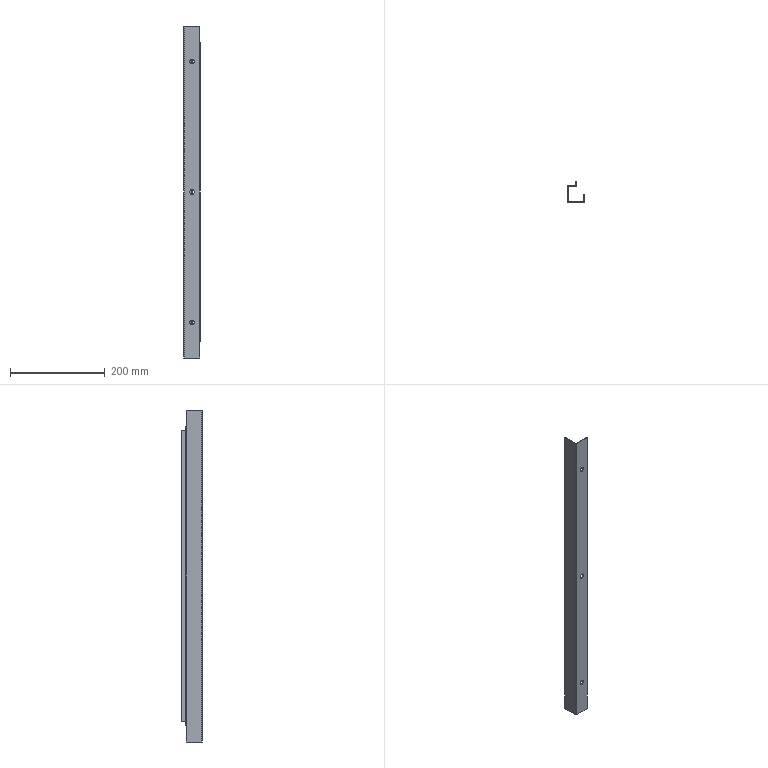Part | SolidWorks | features EdgeFlange 3, ICE 2, FlatPattern 1, LPattern 1, SMBaseFlange 1, SheetMetal 1 | 1 solid | 50 faces | box 35 x 43.5 x 700 mm | volume 106566 mm3 | plane 36 | cylinder 14 | commonest cylinder face diameters 10 x6 3 x4 4.5 x4
STEP:
#1=CARTESIAN_POINT('',(7.75,33.5,307.5));
#2=VERTEX_POINT('',#1);
#3=CARTESIAN_POINT('',(3.25,33.5,307.5));
#4=VERTEX_POINT('',#3);
#5=CARTESIAN_POINT('',(5.5,33.5,307.5));
#6=DIRECTION('',(0.,1.,0.));
#7=DIRECTION('',(-1.,0.,0.));
#8=AXIS2_PLACEMENT_3D('',#5,#6,#7);
#9=CIRCLE('',#8,2.25);
#10=EDGE_CURVE('',#2,#4,#9,.T.);
#11=ORIENTED_EDGE('',*,*,#10,.F.);
#12=CARTESIAN_POINT('',(7.75,35.,307.5));
#13=VERTEX_POINT('',#12);
#14=CARTESIAN_POINT('',(7.75,33.5,307.5));
#15=DIRECTION('',(0.,1.,0.));
#16=VECTOR('',#15,1000.);
#17=LINE('',#14,#16);
#18=EDGE_CURVE('',#2,#13,#17,.T.);
#19=ORIENTED_EDGE('',*,*,#18,.T.);
#20=CARTESIAN_POINT('',(3.25,35.,307.5));
#21=VERTEX_POINT('',#20);
#22=CARTESIAN_POINT('',(5.5,35.,307.5));
#23=DIRECTION('',(0.,1.,0.));
#24=DIRECTION('',(-1.,0.,0.));
#25=AXIS2_PLACEMENT_3D('',#22,#23,#24);
#26=CIRCLE('',#25,2.25);
#27=EDGE_CURVE('',#13,#21,#26,.T.);
#28=ORIENTED_EDGE('',*,*,#27,.T.);
#29=CARTESIAN_POINT('',(3.25,33.5,307.5));
#30=DIRECTION('',(0.,1.,0.));
#31=VECTOR('',#30,1000.);
#32=LINE('',#29,#31);
#33=EDGE_CURVE('',#4,#21,#32,.T.);
#34=ORIENTED_EDGE('',*,*,#33,.F.);
#35=EDGE_LOOP('',(#11,#19,#28,#34));
#36=FACE_OUTER_BOUND('',#35,.T.);
#37=CARTESIAN_POINT('',(5.5,33.5,307.5));
#38=DIRECTION('',(0.,1.,0.));
#39=DIRECTION('',(-1.,0.,0.));
#40=AXIS2_PLACEMENT_3D('',#37,#38,#39);
#41=CYLINDRICAL_SURFACE('',#40,2.25);
#42=ADVANCED_FACE('',(#36),#41,.F.);
#43=CARTESIAN_POINT('',(7.75,33.5,-307.5));
#44=VERTEX_POINT('',#43);
#45=CARTESIAN_POINT('',(3.25,33.5,-307.5));
#46=VERTEX_POINT('',#45);
#47=CARTESIAN_POINT('',(5.5,33.5,-307.5));
#48=DIRECTION('',(0.,1.,0.));
#49=DIRECTION('',(-1.,0.,0.));
#50=AXIS2_PLACEMENT_3D('',#47,#48,#49);
#51=CIRCLE('',#50,2.25);
#52=EDGE_CURVE('',#44,#46,#51,.T.);
#53=ORIENTED_EDGE('',*,*,#52,.F.);
#54=CARTESIAN_POINT('',(7.75,35.,-307.5));
#55=VERTEX_POINT('',#54);
#56=CARTESIAN_POINT('',(7.75,33.5,-307.5));
#57=DIRECTION('',(0.,1.,0.));
#58=VECTOR('',#57,1000.);
#59=LINE('',#56,#58);
#60=EDGE_CURVE('',#44,#55,#59,.T.);
#61=ORIENTED_EDGE('',*,*,#60,.T.);
#62=CARTESIAN_POINT('',(3.25,35.,-307.5));
#63=VERTEX_POINT('',#62);
#64=CARTESIAN_POINT('',(5.5,35.,-307.5));
#65=DIRECTION('',(0.,1.,0.));
#66=DIRECTION('',(-1.,0.,0.));
#67=AXIS2_PLACEMENT_3D('',#64,#65,#66);
#68=CIRCLE('',#67,2.25);
#69=EDGE_CURVE('',#55,#63,#68,.T.);
#70=ORIENTED_EDGE('',*,*,#69,.T.);
#71=CARTESIAN_POINT('',(3.25,33.5,-307.5));
#72=DIRECTION('',(0.,1.,0.));
#73=VECTOR('',#72,1000.);
#74=LINE('',#71,#73);
#75=EDGE_CURVE('',#46,#63,#74,.T.);
#76=ORIENTED_EDGE('',*,*,#75,.F.);
#77=EDGE_LOOP('',(#53,#61,#70,#76));
#78=FACE_OUTER_BOUND('',#77,.T.);
#79=CARTESIAN_POINT('',(5.5,33.5,-307.5));
#80=DIRECTION('',(0.,1.,0.));
#81=DIRECTION('',(-1.,0.,0.));
#82=AXIS2_PLACEMENT_3D('',#79,#80,#81);
#83=CYLINDRICAL_SURFACE('',#82,2.25);
#84=ADVANCED_FACE('',(#78),#83,.F.);
#85=CARTESIAN_POINT('',(17.5,1.5,-270.));
#86=VERTEX_POINT('',#85);
#87=CARTESIAN_POINT('',(17.5,1.5,-280.));
#88=VERTEX_POINT('',#87);
#89=CARTESIAN_POINT('',(17.5,1.5,-275.));
#90=DIRECTION('',(0.,-1.,0.));
#91=DIRECTION('',(0.,0.,-1.));
#92=AXIS2_PLACEMENT_3D('',#89,#90,#91);
#93=CIRCLE('',#92,5.);
#94=EDGE_CURVE('',#86,#88,#93,.T.);
#95=ORIENTED_EDGE('',*,*,#94,.F.);
#96=CARTESIAN_POINT('',(17.5,0.,-270.));
#97=VERTEX_POINT('',#96);
#98=CARTESIAN_POINT('',(17.5,1.5,-270.));
#99=DIRECTION('',(0.,-1.,0.));
#100=VECTOR('',#99,1000.);
#101=LINE('',#98,#100);
#102=EDGE_CURVE('',#86,#97,#101,.T.);
#103=ORIENTED_EDGE('',*,*,#102,.T.);
#104=CARTESIAN_POINT('',(17.5,0.,-280.));
#105=VERTEX_POINT('',#104);
#106=CARTESIAN_POINT('',(17.5,0.,-275.));
#107=DIRECTION('',(0.,-1.,0.));
#108=DIRECTION('',(0.,0.,-1.));
#109=AXIS2_PLACEMENT_3D('',#106,#107,#108);
#110=CIRCLE('',#109,5.);
#111=EDGE_CURVE('',#97,#105,#110,.T.);
#112=ORIENTED_EDGE('',*,*,#111,.T.);
#113=CARTESIAN_POINT('',(17.5,1.5,-280.));
#114=DIRECTION('',(0.,-1.,0.));
#115=VECTOR('',#114,1000.);
#116=LINE('',#113,#115);
#117=EDGE_CURVE('',#88,#105,#116,.T.);
#118=ORIENTED_EDGE('',*,*,#117,.F.);
#119=EDGE_LOOP('',(#95,#103,#112,#118));
#120=FACE_OUTER_BOUND('',#119,.T.);
#121=CARTESIAN_POINT('',(17.5,1.5,-275.));
#122=DIRECTION('',(0.,-1.,0.));
#123=DIRECTION('',(0.,0.,-1.));
#124=AXIS2_PLACEMENT_3D('',#121,#122,#123);
#125=CYLINDRICAL_SURFACE('',#124,5.);
#126=ADVANCED_FACE('',(#120),#125,.F.);
#127=CARTESIAN_POINT('',(17.5,1.5,5.));
#128=VERTEX_POINT('',#127);
#129=CARTESIAN_POINT('',(17.5,1.5,-5.));
#130=VERTEX_POINT('',#129);
#131=CARTESIAN_POINT('',(17.5,1.5,0.));
#132=DIRECTION('',(0.,-1.,0.));
#133=DIRECTION('',(0.,0.,-1.));
#134=AXIS2_PLACEMENT_3D('',#131,#132,#133);
#135=CIRCLE('',#134,5.);
#136=EDGE_CURVE('',#128,#130,#135,.T.);
#137=ORIENTED_EDGE('',*,*,#136,.F.);
#138=CARTESIAN_POINT('',(17.5,0.,5.));
#139=VERTEX_POINT('',#138);
#140=CARTESIAN_POINT('',(17.5,1.5,5.));
#141=DIRECTION('',(0.,-1.,0.));
#142=VECTOR('',#141,1000.);
#143=LINE('',#140,#142);
#144=EDGE_CURVE('',#128,#139,#143,.T.);
#145=ORIENTED_EDGE('',*,*,#144,.T.);
#146=CARTESIAN_POINT('',(17.5,0.,-5.));
#147=VERTEX_POINT('',#146);
#148=CARTESIAN_POINT('',(17.5,0.,0.));
#149=DIRECTION('',(0.,-1.,0.));
#150=DIRECTION('',(0.,0.,-1.));
#151=AXIS2_PLACEMENT_3D('',#148,#149,#150);
#152=CIRCLE('',#151,5.);
#153=EDGE_CURVE('',#139,#147,#152,.T.);
#154=ORIENTED_EDGE('',*,*,#153,.T.);
#155=CARTESIAN_POINT('',(17.5,1.5,-5.));
#156=DIRECTION('',(0.,-1.,0.));
#157=VECTOR('',#156,1000.);
#158=LINE('',#155,#157);
#159=EDGE_CURVE('',#130,#147,#158,.T.);
#160=ORIENTED_EDGE('',*,*,#159,.F.);
#161=EDGE_LOOP('',(#137,#145,#154,#160));
#162=FACE_OUTER_BOUND('',#161,.T.);
#163=CARTESIAN_POINT('',(17.5,1.5,0.));
#164=DIRECTION('',(0.,-1.,0.));
#165=DIRECTION('',(0.,0.,-1.));
#166=AXIS2_PLACEMENT_3D('',#163,#164,#165);
#167=CYLINDRICAL_SURFACE('',#166,5.);
#168=ADVANCED_FACE('',(#162),#167,.F.);
#169=CARTESIAN_POINT('',(17.5,1.5,280.));
#170=VERTEX_POINT('',#169);
#171=CARTESIAN_POINT('',(17.5,1.5,270.));
#172=VERTEX_POINT('',#171);
#173=CARTESIAN_POINT('',(17.5,1.5,275.));
#174=DIRECTION('',(0.,-1.,0.));
#175=DIRECTION('',(0.,0.,-1.));
#176=AXIS2_PLACEMENT_3D('',#173,#174,#175);
#177=CIRCLE('',#176,5.);
#178=EDGE_CURVE('',#170,#172,#177,.T.);
#179=ORIENTED_EDGE('',*,*,#178,.F.);
#180=CARTESIAN_POINT('',(17.5,0.,280.));
#181=VERTEX_POINT('',#180);
#182=CARTESIAN_POINT('',(17.5,1.5,280.));
#183=DIRECTION('',(0.,-1.,0.));
#184=VECTOR('',#183,1000.);
#185=LINE('',#182,#184);
#186=EDGE_CURVE('',#170,#181,#185,.T.);
#187=ORIENTED_EDGE('',*,*,#186,.T.);
#188=CARTESIAN_POINT('',(17.5,0.,270.));
#189=VERTEX_POINT('',#188);
#190=CARTESIAN_POINT('',(17.5,0.,275.));
#191=DIRECTION('',(0.,-1.,0.));
#192=DIRECTION('',(0.,0.,-1.));
#193=AXIS2_PLACEMENT_3D('',#190,#191,#192);
#194=CIRCLE('',#193,5.);
#195=EDGE_CURVE('',#181,#189,#194,.T.);
#196=ORIENTED_EDGE('',*,*,#195,.T.);
#197=CARTESIAN_POINT('',(17.5,1.5,270.));
#198=DIRECTION('',(0.,-1.,0.));
#199=VECTOR('',#198,1000.);
#200=LINE('',#197,#199);
#201=EDGE_CURVE('',#172,#189,#200,.T.);
#202=ORIENTED_EDGE('',*,*,#201,.F.);
#203=EDGE_LOOP('',(#179,#187,#196,#202));
#204=FACE_OUTER_BOUND('',#203,.T.);
#205=CARTESIAN_POINT('',(17.5,1.5,275.));
#206=DIRECTION('',(0.,-1.,0.));
#207=DIRECTION('',(0.,0.,-1.));
#208=AXIS2_PLACEMENT_3D('',#205,#206,#207);
#209=CYLINDRICAL_SURFACE('',#208,5.);
#210=ADVANCED_FACE('',(#204),#209,.F.);
#211=CARTESIAN_POINT('',(33.5,0.,350.));
#212=VERTEX_POINT('',#211);
#213=CARTESIAN_POINT('',(33.5,0.,315.));
#214=VERTEX_POINT('',#213);
#215=CARTESIAN_POINT('',(33.5,0.,350.));
#216=DIRECTION('',(0.,0.,-1.));
#217=VECTOR('',#216,1000.);
#218=LINE('',#215,#217);
#219=EDGE_CURVE('',#212,#214,#218,.T.);
#220=ORIENTED_EDGE('',*,*,#219,.T.);
#221=CARTESIAN_POINT('',(33.5,1.5,315.));
#222=VERTEX_POINT('',#221);
#223=CARTESIAN_POINT('',(33.5,0.,315.));
#224=DIRECTION('',(0.,1.,0.));
#225=VECTOR('',#224,1000.);
#226=LINE('',#223,#225);
#227=EDGE_CURVE('',#214,#222,#226,.T.);
#228=ORIENTED_EDGE('',*,*,#227,.T.);
#229=CARTESIAN_POINT('',(33.5,1.5,350.));
#230=VERTEX_POINT('',#229);
#231=CARTESIAN_POINT('',(33.5,1.5,350.));
#232=DIRECTION('',(0.,0.,-1.));
#233=VECTOR('',#232,1000.);
#234=LINE('',#231,#233);
#235=EDGE_CURVE('',#230,#222,#234,.T.);
#236=ORIENTED_EDGE('',*,*,#235,.F.);
#237=CARTESIAN_POINT('',(33.5,1.5,350.));
#238=DIRECTION('',(0.,-1.,0.));
#239=VECTOR('',#238,1000.);
#240=LINE('',#237,#239);
#241=EDGE_CURVE('',#230,#212,#240,.T.);
#242=ORIENTED_EDGE('',*,*,#241,.T.);
#243=EDGE_LOOP('',(#220,#228,#236,#242));
#244=FACE_OUTER_BOUND('',#243,.T.);
#245=CARTESIAN_POINT('',(33.5,1.5,350.));
#246=DIRECTION('',(1.,0.,0.));
#247=DIRECTION('',(0.,0.,-1.));
#248=AXIS2_PLACEMENT_3D('',#245,#246,#247);
#249=PLANE('',#248);
#250=ADVANCED_FACE('',(#244),#249,.T.);
#251=CARTESIAN_POINT('',(17.,33.5,-306.5));
#252=VERTEX_POINT('',#251);
#253=CARTESIAN_POINT('',(17.,35.,-306.5));
#254=VERTEX_POINT('',#253);
#255=CARTESIAN_POINT('',(17.,33.5,-306.5));
#256=DIRECTION('',(0.,1.,0.));
#257=VECTOR('',#256,1000.);
#258=LINE('',#255,#257);
#259=EDGE_CURVE('',#252,#254,#258,.T.);
#260=ORIENTED_EDGE('',*,*,#259,.F.);
#261=CARTESIAN_POINT('',(17.,33.5,-315.));
#262=VERTEX_POINT('',#261);
#263=CARTESIAN_POINT('',(17.,33.5,-315.));
#264=DIRECTION('',(0.,0.,-1.));
#265=VECTOR('',#264,1000.);
#266=LINE('',#263,#265);
#267=EDGE_CURVE('',#252,#262,#266,.T.);
#268=ORIENTED_EDGE('',*,*,#267,.T.);
#269=CARTESIAN_POINT('',(17.,35.,-315.));
#270=VERTEX_POINT('',#269);
#271=CARTESIAN_POINT('',(17.,35.,-315.));
#272=DIRECTION('',(0.,-1.,0.));
#273=VECTOR('',#272,1000.);
#274=LINE('',#271,#273);
#275=EDGE_CURVE('',#270,#262,#274,.T.);
#276=ORIENTED_EDGE('',*,*,#275,.F.);
#277=CARTESIAN_POINT('',(17.,35.,-315.));
#278=DIRECTION('',(0.,0.,-1.));
#279=VECTOR('',#278,1000.);
#280=LINE('',#277,#279);
#281=EDGE_CURVE('',#254,#270,#280,.T.);
#282=ORIENTED_EDGE('',*,*,#281,.F.);
#283=EDGE_LOOP('',(#260,#268,#276,#282));
#284=FACE_OUTER_BOUND('',#283,.T.);
#285=CARTESIAN_POINT('',(17.,35.,-315.));
#286=DIRECTION('',(-1.,0.,0.));
#287=DIRECTION('',(0.,-1.,0.));
#288=AXIS2_PLACEMENT_3D('',#285,#286,#287);
#289=PLANE('',#288);
#290=ADVANCED_FACE('',(#284),#289,.F.);
#291=CARTESIAN_POINT('',(0.,33.5,-315.));
#292=VERTEX_POINT('',#291);
#293=CARTESIAN_POINT('',(0.,33.5,-350.));
#294=VERTEX_POINT('',#293);
#295=CARTESIAN_POINT('',(0.,33.5,350.));
#296=DIRECTION('',(0.,0.,-1.));
#297=VECTOR('',#296,1000.);
#298=LINE('',#295,#297);
#299=EDGE_CURVE('',#292,#294,#298,.T.);
#300=ORIENTED_EDGE('',*,*,#299,.F.);
#301=CARTESIAN_POINT('',(1.5,33.5,-315.));
#302=VERTEX_POINT('',#301);
#303=CARTESIAN_POINT('',(0.,33.5,-315.));
#304=DIRECTION('',(1.,0.,0.));
#305=VECTOR('',#304,1000.);
#306=LINE('',#303,#305);
#307=EDGE_CURVE('',#292,#302,#306,.T.);
#308=ORIENTED_EDGE('',*,*,#307,.T.);
#309=CARTESIAN_POINT('',(1.5,33.5,-350.));
#310=VERTEX_POINT('',#309);
#311=CARTESIAN_POINT('',(1.5,33.5,350.));
#312=DIRECTION('',(0.,0.,-1.));
#313=VECTOR('',#312,1000.);
#314=LINE('',#311,#313);
#315=EDGE_CURVE('',#302,#310,#314,.T.);
#316=ORIENTED_EDGE('',*,*,#315,.T.);
#317=CARTESIAN_POINT('',(0.,33.5,-350.));
#318=DIRECTION('',(1.,0.,0.));
#319=VECTOR('',#318,1000.);
#320=LINE('',#317,#319);
#321=EDGE_CURVE('',#294,#310,#320,.T.);
#322=ORIENTED_EDGE('',*,*,#321,.F.);
#323=EDGE_LOOP('',(#300,#308,#316,#322));
#324=FACE_OUTER_BOUND('',#323,.T.);
#325=CARTESIAN_POINT('',(0.,33.5,350.));
#326=DIRECTION('',(0.,1.,0.));
#327=DIRECTION('',(0.,0.,1.));
#328=AXIS2_PLACEMENT_3D('',#325,#326,#327);
#329=PLANE('',#328);
#330=ADVANCED_FACE('',(#324),#329,.T.);
#331=CARTESIAN_POINT('',(1.5,1.5,350.));
#332=VERTEX_POINT('',#331);
#333=CARTESIAN_POINT('',(0.,1.5,350.));
#334=VERTEX_POINT('',#333);
#335=CARTESIAN_POINT('',(1.5,1.5,350.));
#336=DIRECTION('',(-1.,0.,0.));
#337=VECTOR('',#336,1000.);
#338=LINE('',#335,#337);
#339=EDGE_CURVE('',#332,#334,#338,.T.);
#340=ORIENTED_EDGE('',*,*,#339,.F.);
#341=CARTESIAN_POINT('',(1.5,33.5,350.));
#342=VERTEX_POINT('',#341);
#343=CARTESIAN_POINT('',(1.5,33.5,350.));
#344=DIRECTION('',(0.,-1.,0.));
#345=VECTOR('',#344,1000.);
#346=LINE('',#343,#345);
#347=EDGE_CURVE('',#342,#332,#346,.T.);
#348=ORIENTED_EDGE('',*,*,#347,.F.);
#349=CARTESIAN_POINT('',(0.,33.5,350.));
#350=VERTEX_POINT('',#349);
#351=CARTESIAN_POINT('',(0.,33.5,350.));
#352=DIRECTION('',(1.,0.,0.));
#353=VECTOR('',#352,1000.);
#354=LINE('',#351,#353);
#355=EDGE_CURVE('',#350,#342,#354,.T.);
#356=ORIENTED_EDGE('',*,*,#355,.F.);
#357=CARTESIAN_POINT('',(0.,33.5,350.));
#358=DIRECTION('',(0.,-1.,0.));
#359=VECTOR('',#358,1000.);
#360=LINE('',#357,#359);
#361=EDGE_CURVE('',#350,#334,#360,.T.);
#362=ORIENTED_EDGE('',*,*,#361,.T.);
#363=EDGE_LOOP('',(#340,#348,#356,#362));
#364=FACE_OUTER_BOUND('',#363,.T.);
#365=CARTESIAN_POINT('',(1.5,1.5,350.));
#366=DIRECTION('',(0.,0.,1.));
#367=DIRECTION('',(1.,0.,0.));
#368=AXIS2_PLACEMENT_3D('',#365,#366,#367);
#369=PLANE('',#368);
#370=ADVANCED_FACE('',(#364),#369,.T.);
#371=CARTESIAN_POINT('',(1.5,0.,350.));
#372=VERTEX_POINT('',#371);
#373=CARTESIAN_POINT('',(1.5,1.5,350.));
#374=DIRECTION('',(0.,-1.,0.));
#375=VECTOR('',#374,1000.);
#376=LINE('',#373,#375);
#377=EDGE_CURVE('',#332,#372,#376,.T.);
#378=ORIENTED_EDGE('',*,*,#377,.F.);
#379=ORIENTED_EDGE('',*,*,#339,.T.);
#380=CARTESIAN_POINT('',(1.5,1.5,350.));
#381=DIRECTION('',(0.,0.,1.));
#382=DIRECTION('',(-1.,0.,0.));
#383=AXIS2_PLACEMENT_3D('',#380,#381,#382);
#384=CIRCLE('',#383,1.5);
#385=EDGE_CURVE('',#334,#372,#384,.T.);
#386=ORIENTED_EDGE('',*,*,#385,.T.);
#387=EDGE_LOOP('',(#378,#379,#386));
#388=FACE_OUTER_BOUND('',#387,.T.);
#389=CARTESIAN_POINT('',(1.5,1.5,350.));
#390=DIRECTION('',(0.,0.,1.));
#391=DIRECTION('',(1.,0.,0.));
#392=AXIS2_PLACEMENT_3D('',#389,#390,#391);
#393=PLANE('',#392);
#394=ADVANCED_FACE('',(#388),#393,.T.);
#395=CARTESIAN_POINT('',(1.5,1.5,-350.));
#396=VERTEX_POINT('',#395);
#397=CARTESIAN_POINT('',(1.5,0.,-350.));
#398=VERTEX_POINT('',#397);
#399=CARTESIAN_POINT('',(1.5,1.5,-350.));
#400=DIRECTION('',(0.,-1.,0.));
#401=VECTOR('',#400,1000.);
#402=LINE('',#399,#401);
#403=EDGE_CURVE('',#396,#398,#402,.T.);
#404=ORIENTED_EDGE('',*,*,#403,.F.);
#405=CARTESIAN_POINT('',(33.5,1.5,-350.));
#406=VERTEX_POINT('',#405);
#407=CARTESIAN_POINT('',(0.,1.5,-350.));
#408=DIRECTION('',(1.,0.,0.));
#409=VECTOR('',#408,1000.);
#410=LINE('',#407,#409);
#411=EDGE_CURVE('',#396,#406,#410,.T.);
#412=ORIENTED_EDGE('',*,*,#411,.T.);
#413=CARTESIAN_POINT('',(33.5,0.,-350.));
#414=VERTEX_POINT('',#413);
#415=CARTESIAN_POINT('',(33.5,1.5,-350.));
#416=DIRECTION('',(0.,-1.,0.));
#417=VECTOR('',#416,1000.);
#418=LINE('',#415,#417);
#419=EDGE_CURVE('',#406,#414,#418,.T.);
#420=ORIENTED_EDGE('',*,*,#419,.T.);
#421=CARTESIAN_POINT('',(0.,0.,-350.));
#422=DIRECTION('',(1.,0.,0.));
#423=VECTOR('',#422,1000.);
#424=LINE('',#421,#423);
#425=EDGE_CURVE('',#398,#414,#424,.T.);
#426=ORIENTED_EDGE('',*,*,#425,.F.);
#427=EDGE_LOOP('',(#404,#412,#420,#426));
#428=FACE_OUTER_BOUND('',#427,.T.);
#429=CARTESIAN_POINT('',(1.5,1.5,-350.));
#430=DIRECTION('',(0.,0.,-1.));
#431=DIRECTION('',(-1.,0.,0.));
#432=AXIS2_PLACEMENT_3D('',#429,#430,#431);
#433=PLANE('',#432);
#434=ADVANCED_FACE('',(#428),#433,.T.);
#435=CARTESIAN_POINT('',(0.,1.5,-350.));
#436=VERTEX_POINT('',#435);
#437=CARTESIAN_POINT('',(1.5,1.5,-350.));
#438=DIRECTION('',(-1.,0.,0.));
#439=VECTOR('',#438,1000.);
#440=LINE('',#437,#439);
#441=EDGE_CURVE('',#396,#436,#440,.T.);
#442=ORIENTED_EDGE('',*,*,#441,.F.);
#443=ORIENTED_EDGE('',*,*,#403,.T.);
#444=CARTESIAN_POINT('',(1.5,1.5,-350.));
#445=DIRECTION('',(0.,0.,1.));
#446=DIRECTION('',(-1.,0.,0.));
#447=AXIS2_PLACEMENT_3D('',#444,#445,#446);
#448=CIRCLE('',#447,1.5);
#449=EDGE_CURVE('',#436,#398,#448,.T.);
#450=ORIENTED_EDGE('',*,*,#449,.F.);
#451=EDGE_LOOP('',(#442,#443,#450));
#452=FACE_OUTER_BOUND('',#451,.T.);
#453=CARTESIAN_POINT('',(1.5,1.5,-350.));
#454=DIRECTION('',(0.,0.,-1.));
#455=DIRECTION('',(-1.,0.,0.));
#456=AXIS2_PLACEMENT_3D('',#453,#454,#455);
#457=PLANE('',#456);
#458=ADVANCED_FACE('',(#452),#457,.T.);
#459=CARTESIAN_POINT('',(17.5,0.,0.));
#460=DIRECTION('',(0.,-1.,0.));
#461=DIRECTION('',(0.,0.,-1.));
#462=AXIS2_PLACEMENT_3D('',#459,#460,#461);
#463=CIRCLE('',#462,5.);
#464=EDGE_CURVE('',#147,#139,#463,.T.);
#465=ORIENTED_EDGE('',*,*,#464,.F.);
#466=ORIENTED_EDGE('',*,*,#153,.F.);
#467=EDGE_LOOP('',(#465,#466));
#468=FACE_BOUND('',#467,.T.);
#469=CARTESIAN_POINT('',(17.5,0.,275.));
#470=DIRECTION('',(0.,-1.,0.));
#471=DIRECTION('',(0.,0.,-1.));
#472=AXIS2_PLACEMENT_3D('',#469,#470,#471);
#473=CIRCLE('',#472,5.);
#474=EDGE_CURVE('',#189,#181,#473,.T.);
#475=ORIENTED_EDGE('',*,*,#474,.F.);
#476=ORIENTED_EDGE('',*,*,#195,.F.);
#477=EDGE_LOOP('',(#475,#476));
#478=FACE_BOUND('',#477,.T.);
#479=ORIENTED_EDGE('',*,*,#425,.T.);
#480=CARTESIAN_POINT('',(33.5,0.,-315.));
#481=VERTEX_POINT('',#480);
#482=CARTESIAN_POINT('',(33.5,0.,350.));
#483=DIRECTION('',(0.,0.,-1.));
#484=VECTOR('',#483,1000.);
#485=LINE('',#482,#484);
#486=EDGE_CURVE('',#481,#414,#485,.T.);
#487=ORIENTED_EDGE('',*,*,#486,.F.);
#488=CARTESIAN_POINT('',(33.5,0.,315.));
#489=DIRECTION('',(0.,0.,-1.));
#490=VECTOR('',#489,1000.);
#491=LINE('',#488,#490);
#492=EDGE_CURVE('',#214,#481,#491,.T.);
#493=ORIENTED_EDGE('',*,*,#492,.F.);
#494=ORIENTED_EDGE('',*,*,#219,.F.);
#495=CARTESIAN_POINT('',(0.,0.,350.));
#496=DIRECTION('',(1.,0.,0.));
#497=VECTOR('',#496,1000.);
#498=LINE('',#495,#497);
#499=EDGE_CURVE('',#372,#212,#498,.T.);
#500=ORIENTED_EDGE('',*,*,#499,.F.);
#501=CARTESIAN_POINT('',(1.5,0.,350.));
#502=DIRECTION('',(0.,0.,-1.));
#503=VECTOR('',#502,1000.);
#504=LINE('',#501,#503);
#505=EDGE_CURVE('',#372,#398,#504,.T.);
#506=ORIENTED_EDGE('',*,*,#505,.T.);
#507=EDGE_LOOP('',(#479,#487,#493,#494,#500,#506));
#508=FACE_OUTER_BOUND('',#507,.T.);
#509=CARTESIAN_POINT('',(17.5,0.,-275.));
#510=DIRECTION('',(0.,-1.,0.));
#511=DIRECTION('',(0.,0.,-1.));
#512=AXIS2_PLACEMENT_3D('',#509,#510,#511);
#513=CIRCLE('',#512,5.);
#514=EDGE_CURVE('',#105,#97,#513,.T.);
#515=ORIENTED_EDGE('',*,*,#514,.F.);
#516=ORIENTED_EDGE('',*,*,#111,.F.);
#517=EDGE_LOOP('',(#515,#516));
#518=FACE_BOUND('',#517,.T.);
#519=CARTESIAN_POINT('',(0.,0.,350.));
#520=DIRECTION('',(0.,1.,0.));
#521=DIRECTION('',(0.,0.,1.));
#522=AXIS2_PLACEMENT_3D('',#519,#520,#521);
#523=PLANE('',#522);
#524=ADVANCED_FACE('',(#468,#478,#508,#518),#523,.F.);
#525=CARTESIAN_POINT('',(33.5,1.5,-315.));
#526=VERTEX_POINT('',#525);
#527=CARTESIAN_POINT('',(33.5,0.,-315.));
#528=DIRECTION('',(0.,1.,0.));
#529=VECTOR('',#528,1000.);
#530=LINE('',#527,#529);
#531=EDGE_CURVE('',#481,#526,#530,.T.);
#532=ORIENTED_EDGE('',*,*,#531,.F.);
#533=ORIENTED_EDGE('',*,*,#486,.T.);
#534=ORIENTED_EDGE('',*,*,#419,.F.);
#535=CARTESIAN_POINT('',(33.5,1.5,350.));
#536=DIRECTION('',(0.,0.,-1.));
#537=VECTOR('',#536,1000.);
#538=LINE('',#535,#537);
#539=EDGE_CURVE('',#526,#406,#538,.T.);
#540=ORIENTED_EDGE('',*,*,#539,.F.);
#541=EDGE_LOOP('',(#532,#533,#534,#540));
#542=FACE_OUTER_BOUND('',#541,.T.);
#543=CARTESIAN_POINT('',(33.5,1.5,350.));
#544=DIRECTION('',(1.,0.,0.));
#545=DIRECTION('',(0.,0.,-1.));
#546=AXIS2_PLACEMENT_3D('',#543,#544,#545);
#547=PLANE('',#546);
#548=ADVANCED_FACE('',(#542),#547,.T.);
#549=CARTESIAN_POINT('',(17.5,1.5,0.));
#550=DIRECTION('',(0.,-1.,0.));
#551=DIRECTION('',(0.,0.,-1.));
#552=AXIS2_PLACEMENT_3D('',#549,#550,#551);
#553=CIRCLE('',#552,5.);
#554=EDGE_CURVE('',#130,#128,#553,.T.);
#555=ORIENTED_EDGE('',*,*,#554,.T.);
#556=ORIENTED_EDGE('',*,*,#136,.T.);
#557=EDGE_LOOP('',(#555,#556));
#558=FACE_BOUND('',#557,.T.);
#559=CARTESIAN_POINT('',(17.5,1.5,275.));
#560=DIRECTION('',(0.,-1.,0.));
#561=DIRECTION('',(0.,0.,-1.));
#562=AXIS2_PLACEMENT_3D('',#559,#560,#561);
#563=CIRCLE('',#562,5.);
#564=EDGE_CURVE('',#172,#170,#563,.T.);
#565=ORIENTED_EDGE('',*,*,#564,.T.);
#566=ORIENTED_EDGE('',*,*,#178,.T.);
#567=EDGE_LOOP('',(#565,#566));
#568=FACE_BOUND('',#567,.T.);
#569=ORIENTED_EDGE('',*,*,#411,.F.);
#570=CARTESIAN_POINT('',(1.5,1.5,350.));
#571=DIRECTION('',(0.,0.,-1.));
#572=VECTOR('',#571,1000.);
#573=LINE('',#570,#572);
#574=EDGE_CURVE('',#332,#396,#573,.T.);
#575=ORIENTED_EDGE('',*,*,#574,.F.);
#576=CARTESIAN_POINT('',(0.,1.5,350.));
#577=DIRECTION('',(1.,0.,0.));
#578=VECTOR('',#577,1000.);
#579=LINE('',#576,#578);
#580=EDGE_CURVE('',#332,#230,#579,.T.);
#581=ORIENTED_EDGE('',*,*,#580,.T.);
#582=ORIENTED_EDGE('',*,*,#235,.T.);
#583=CARTESIAN_POINT('',(33.5,1.5,315.));
#584=DIRECTION('',(0.,0.,-1.));
#585=VECTOR('',#584,1000.);
#586=LINE('',#583,#585);
#587=EDGE_CURVE('',#222,#526,#586,.T.);
#588=ORIENTED_EDGE('',*,*,#587,.T.);
#589=ORIENTED_EDGE('',*,*,#539,.T.);
#590=EDGE_LOOP('',(#569,#575,#581,#582,#588,#589));
#591=FACE_OUTER_BOUND('',#590,.T.);
#592=CARTESIAN_POINT('',(17.5,1.5,-275.));
#593=DIRECTION('',(0.,-1.,0.));
#594=DIRECTION('',(0.,0.,-1.));
#595=AXIS2_PLACEMENT_3D('',#592,#593,#594);
#596=CIRCLE('',#595,5.);
#597=EDGE_CURVE('',#88,#86,#596,.T.);
#598=ORIENTED_EDGE('',*,*,#597,.T.);
#599=ORIENTED_EDGE('',*,*,#94,.T.);
#600=EDGE_LOOP('',(#598,#599));
#601=FACE_BOUND('',#600,.T.);
#602=CARTESIAN_POINT('',(0.,1.5,350.));
#603=DIRECTION('',(0.,1.,0.));
#604=DIRECTION('',(0.,0.,1.));
#605=AXIS2_PLACEMENT_3D('',#602,#603,#604);
#606=PLANE('',#605);
#607=ADVANCED_FACE('',(#558,#568,#591,#601),#606,.T.);
#608=CARTESIAN_POINT('',(1.5,33.5,-350.));
#609=DIRECTION('',(0.,-1.,0.));
#610=VECTOR('',#609,1000.);
#611=LINE('',#608,#610);
#612=EDGE_CURVE('',#310,#396,#611,.T.);
#613=ORIENTED_EDGE('',*,*,#612,.F.);
#614=ORIENTED_EDGE('',*,*,#315,.F.);
#615=CARTESIAN_POINT('',(1.5,33.5,315.));
#616=VERTEX_POINT('',#615);
#617=CARTESIAN_POINT('',(1.5,33.5,315.));
#618=DIRECTION('',(0.,0.,1.));
#619=VECTOR('',#618,1000.);
#620=LINE('',#617,#619);
#621=EDGE_CURVE('',#302,#616,#620,.T.);
#622=ORIENTED_EDGE('',*,*,#621,.T.);
#623=CARTESIAN_POINT('',(1.5,33.5,350.));
#624=DIRECTION('',(0.,0.,-1.));
#625=VECTOR('',#624,1000.);
#626=LINE('',#623,#625);
#627=EDGE_CURVE('',#342,#616,#626,.T.);
#628=ORIENTED_EDGE('',*,*,#627,.F.);
#629=ORIENTED_EDGE('',*,*,#347,.T.);
#630=ORIENTED_EDGE('',*,*,#574,.T.);
#631=EDGE_LOOP('',(#613,#614,#622,#628,#629,#630));
#632=FACE_OUTER_BOUND('',#631,.T.);
#633=CARTESIAN_POINT('',(1.5,33.5,350.));
#634=DIRECTION('',(1.,0.,0.));
#635=DIRECTION('',(0.,1.,0.));
#636=AXIS2_PLACEMENT_3D('',#633,#634,#635);
#637=PLANE('',#636);
#638=ADVANCED_FACE('',(#632),#637,.T.);
#639=CARTESIAN_POINT('',(0.,33.5,315.));
#640=VERTEX_POINT('',#639);
#641=CARTESIAN_POINT('',(0.,33.5,315.));
#642=DIRECTION('',(1.,0.,0.));
#643=VECTOR('',#642,1000.);
#644=LINE('',#641,#643);
#645=EDGE_CURVE('',#640,#616,#644,.T.);
#646=ORIENTED_EDGE('',*,*,#645,.F.);
#647=CARTESIAN_POINT('',(0.,33.5,350.));
#648=DIRECTION('',(0.,0.,-1.));
#649=VECTOR('',#648,1000.);
#650=LINE('',#647,#649);
#651=EDGE_CURVE('',#350,#640,#650,.T.);
#652=ORIENTED_EDGE('',*,*,#651,.F.);
#653=ORIENTED_EDGE('',*,*,#355,.T.);
#654=ORIENTED_EDGE('',*,*,#627,.T.);
#655=EDGE_LOOP('',(#646,#652,#653,#654));
#656=FACE_OUTER_BOUND('',#655,.T.);
#657=CARTESIAN_POINT('',(0.,33.5,350.));
#658=DIRECTION('',(0.,1.,0.));
#659=DIRECTION('',(0.,0.,1.));
#660=AXIS2_PLACEMENT_3D('',#657,#658,#659);
#661=PLANE('',#660);
#662=ADVANCED_FACE('',(#656),#661,.T.);
#663=CARTESIAN_POINT('',(0.,33.5,-350.));
#664=DIRECTION('',(0.,-1.,0.));
#665=VECTOR('',#664,1000.);
#666=LINE('',#663,#665);
#667=EDGE_CURVE('',#294,#436,#666,.T.);
#668=ORIENTED_EDGE('',*,*,#667,.T.);
#669=CARTESIAN_POINT('',(0.,1.5,350.));
#670=DIRECTION('',(0.,0.,-1.));
#671=VECTOR('',#670,1000.);
#672=LINE('',#669,#671);
#673=EDGE_CURVE('',#334,#436,#672,.T.);
#674=ORIENTED_EDGE('',*,*,#673,.F.);
#675=ORIENTED_EDGE('',*,*,#361,.F.);
#676=ORIENTED_EDGE('',*,*,#651,.T.);
#677=CARTESIAN_POINT('',(0.,33.5,315.));
#678=DIRECTION('',(0.,0.,1.));
#679=VECTOR('',#678,1000.);
#680=LINE('',#677,#679);
#681=EDGE_CURVE('',#292,#640,#680,.T.);
#682=ORIENTED_EDGE('',*,*,#681,.F.);
#683=ORIENTED_EDGE('',*,*,#299,.T.);
#684=EDGE_LOOP('',(#668,#674,#675,#676,#682,#683));
#685=FACE_OUTER_BOUND('',#684,.T.);
#686=CARTESIAN_POINT('',(0.,33.5,350.));
#687=DIRECTION('',(1.,0.,0.));
#688=DIRECTION('',(0.,1.,0.));
#689=AXIS2_PLACEMENT_3D('',#686,#687,#688);
#690=PLANE('',#689);
#691=ADVANCED_FACE('',(#685),#690,.F.);
#692=ORIENTED_EDGE('',*,*,#449,.T.);
#693=ORIENTED_EDGE('',*,*,#505,.F.);
#694=ORIENTED_EDGE('',*,*,#385,.F.);
#695=ORIENTED_EDGE('',*,*,#673,.T.);
#696=EDGE_LOOP('',(#692,#693,#694,#695));
#697=FACE_OUTER_BOUND('',#696,.T.);
#698=CARTESIAN_POINT('',(1.5,1.5,350.));
#699=DIRECTION('',(0.,0.,-1.));
#700=DIRECTION('',(-1.,0.,0.));
#701=AXIS2_PLACEMENT_3D('',#698,#699,#700);
#702=CYLINDRICAL_SURFACE('',#701,1.5);
#703=ADVANCED_FACE('',(#697),#702,.T.);
#704=ORIENTED_EDGE('',*,*,#499,.T.);
#705=ORIENTED_EDGE('',*,*,#241,.F.);
#706=ORIENTED_EDGE('',*,*,#580,.F.);
#707=ORIENTED_EDGE('',*,*,#377,.T.);
#708=EDGE_LOOP('',(#704,#705,#706,#707));
#709=FACE_OUTER_BOUND('',#708,.T.);
#710=CARTESIAN_POINT('',(1.5,1.5,350.));
#711=DIRECTION('',(0.,0.,-1.));
#712=DIRECTION('',(-1.,0.,0.));
#713=AXIS2_PLACEMENT_3D('',#710,#711,#712);
#714=PLANE('',#713);
#715=ADVANCED_FACE('',(#709),#714,.F.);
#716=ORIENTED_EDGE('',*,*,#612,.T.);
#717=ORIENTED_EDGE('',*,*,#441,.T.);
#718=ORIENTED_EDGE('',*,*,#667,.F.);
#719=ORIENTED_EDGE('',*,*,#321,.T.);
#720=EDGE_LOOP('',(#716,#717,#718,#719));
#721=FACE_OUTER_BOUND('',#720,.T.);
#722=CARTESIAN_POINT('',(1.5,1.5,-350.));
#723=DIRECTION('',(0.,0.,-1.));
#724=DIRECTION('',(-1.,0.,0.));
#725=AXIS2_PLACEMENT_3D('',#722,#723,#724);
#726=PLANE('',#725);
#727=ADVANCED_FACE('',(#721),#726,.T.);
#728=CARTESIAN_POINT('',(1.5,35.,315.));
#729=VERTEX_POINT('',#728);
#730=CARTESIAN_POINT('',(1.5,33.5,315.));
#731=DIRECTION('',(0.,0.,-1.));
#732=DIRECTION('',(-1.,0.,0.));
#733=AXIS2_PLACEMENT_3D('',#730,#731,#732);
#734=CIRCLE('',#733,1.5);
#735=EDGE_CURVE('',#640,#729,#734,.T.);
#736=ORIENTED_EDGE('',*,*,#735,.F.);
#737=ORIENTED_EDGE('',*,*,#645,.T.);
#738=CARTESIAN_POINT('',(1.5,35.,315.));
#739=DIRECTION('',(0.,-1.,0.));
#740=VECTOR('',#739,1000.);
#741=LINE('',#738,#740);
#742=EDGE_CURVE('',#729,#616,#741,.T.);
#743=ORIENTED_EDGE('',*,*,#742,.F.);
#744=EDGE_LOOP('',(#736,#737,#743));
#745=FACE_OUTER_BOUND('',#744,.T.);
#746=CARTESIAN_POINT('',(0.,33.5,315.));
#747=DIRECTION('',(0.,0.,1.));
#748=DIRECTION('',(1.,0.,0.));
#749=AXIS2_PLACEMENT_3D('',#746,#747,#748);
#750=PLANE('',#749);
#751=ADVANCED_FACE('',(#745),#750,.T.);
#752=CARTESIAN_POINT('',(1.5,35.,-315.));
#753=VERTEX_POINT('',#752);
#754=CARTESIAN_POINT('',(1.5,33.5,-315.));
#755=DIRECTION('',(0.,0.,-1.));
#756=DIRECTION('',(-1.,0.,0.));
#757=AXIS2_PLACEMENT_3D('',#754,#755,#756);
#758=CIRCLE('',#757,1.5);
#759=EDGE_CURVE('',#292,#753,#758,.T.);
#760=ORIENTED_EDGE('',*,*,#759,.F.);
#761=ORIENTED_EDGE('',*,*,#681,.T.);
#762=ORIENTED_EDGE('',*,*,#735,.T.);
#763=CARTESIAN_POINT('',(1.5,35.,315.));
#764=DIRECTION('',(0.,0.,1.));
#765=VECTOR('',#764,1000.);
#766=LINE('',#763,#765);
#767=EDGE_CURVE('',#753,#729,#766,.T.);
#768=ORIENTED_EDGE('',*,*,#767,.F.);
#769=EDGE_LOOP('',(#760,#761,#762,#768));
#770=FACE_OUTER_BOUND('',#769,.T.);
#771=CARTESIAN_POINT('',(1.5,33.5,-315.));
#772=DIRECTION('',(0.,0.,-1.));
#773=DIRECTION('',(-1.,0.,0.));
#774=AXIS2_PLACEMENT_3D('',#771,#772,#773);
#775=CYLINDRICAL_SURFACE('',#774,1.5);
#776=ADVANCED_FACE('',(#770),#775,.T.);
#777=ORIENTED_EDGE('',*,*,#307,.F.);
#778=ORIENTED_EDGE('',*,*,#759,.T.);
#779=CARTESIAN_POINT('',(1.5,35.,-315.));
#780=DIRECTION('',(0.,-1.,0.));
#781=VECTOR('',#780,1000.);
#782=LINE('',#779,#781);
#783=EDGE_CURVE('',#753,#302,#782,.T.);
#784=ORIENTED_EDGE('',*,*,#783,.T.);
#785=EDGE_LOOP('',(#777,#778,#784));
#786=FACE_OUTER_BOUND('',#785,.T.);
#787=CARTESIAN_POINT('',(0.,33.5,-315.));
#788=DIRECTION('',(0.,0.,1.));
#789=DIRECTION('',(1.,0.,0.));
#790=AXIS2_PLACEMENT_3D('',#787,#788,#789);
#791=PLANE('',#790);
#792=ADVANCED_FACE('',(#786),#791,.F.);
#793=CARTESIAN_POINT('',(17.,33.5,315.));
#794=VERTEX_POINT('',#793);
#795=CARTESIAN_POINT('',(17.,33.5,315.));
#796=DIRECTION('',(1.,0.,0.));
#797=VECTOR('',#796,1000.);
#798=LINE('',#795,#797);
#799=EDGE_CURVE('',#616,#794,#798,.T.);
#800=ORIENTED_EDGE('',*,*,#799,.T.);
#801=CARTESIAN_POINT('',(17.,35.,315.));
#802=VERTEX_POINT('',#801);
#803=CARTESIAN_POINT('',(17.,35.,315.));
#804=DIRECTION('',(0.,-1.,0.));
#805=VECTOR('',#804,1000.);
#806=LINE('',#803,#805);
#807=EDGE_CURVE('',#802,#794,#806,.T.);
#808=ORIENTED_EDGE('',*,*,#807,.F.);
#809=CARTESIAN_POINT('',(17.,35.,315.));
#810=DIRECTION('',(1.,0.,0.));
#811=VECTOR('',#810,1000.);
#812=LINE('',#809,#811);
#813=EDGE_CURVE('',#729,#802,#812,.T.);
#814=ORIENTED_EDGE('',*,*,#813,.F.);
#815=ORIENTED_EDGE('',*,*,#742,.T.);
#816=EDGE_LOOP('',(#800,#808,#814,#815));
#817=FACE_OUTER_BOUND('',#816,.T.);
#818=CARTESIAN_POINT('',(17.,35.,315.));
#819=DIRECTION('',(0.,0.,-1.));
#820=DIRECTION('',(-1.,0.,0.));
#821=AXIS2_PLACEMENT_3D('',#818,#819,#820);
#822=PLANE('',#821);
#823=ADVANCED_FACE('',(#817),#822,.F.);
#824=CARTESIAN_POINT('',(17.,33.5,306.5));
#825=VERTEX_POINT('',#824);
#826=CARTESIAN_POINT('',(17.,33.5,-315.));
#827=DIRECTION('',(0.,0.,-1.));
#828=VECTOR('',#827,1000.);
#829=LINE('',#826,#828);
#830=EDGE_CURVE('',#794,#825,#829,.T.);
#831=ORIENTED_EDGE('',*,*,#830,.T.);
#832=CARTESIAN_POINT('',(17.,35.,306.5));
#833=VERTEX_POINT('',#832);
#834=CARTESIAN_POINT('',(17.,33.5,306.5));
#835=DIRECTION('',(0.,1.,0.));
#836=VECTOR('',#835,1000.);
#837=LINE('',#834,#836);
#838=EDGE_CURVE('',#825,#833,#837,.T.);
#839=ORIENTED_EDGE('',*,*,#838,.T.);
#840=CARTESIAN_POINT('',(17.,35.,-315.));
#841=DIRECTION('',(0.,0.,-1.));
#842=VECTOR('',#841,1000.);
#843=LINE('',#840,#842);
#844=EDGE_CURVE('',#802,#833,#843,.T.);
#845=ORIENTED_EDGE('',*,*,#844,.F.);
#846=ORIENTED_EDGE('',*,*,#807,.T.);
#847=EDGE_LOOP('',(#831,#839,#845,#846));
#848=FACE_OUTER_BOUND('',#847,.T.);
#849=CARTESIAN_POINT('',(17.,35.,-315.));
#850=DIRECTION('',(-1.,0.,0.));
#851=DIRECTION('',(0.,-1.,0.));
#852=AXIS2_PLACEMENT_3D('',#849,#850,#851);
#853=PLANE('',#852);
#854=ADVANCED_FACE('',(#848),#853,.F.);
#855=CARTESIAN_POINT('',(1.5,33.5,-315.));
#856=DIRECTION('',(-1.,0.,0.));
#857=VECTOR('',#856,1000.);
#858=LINE('',#855,#857);
#859=EDGE_CURVE('',#262,#302,#858,.T.);
#860=ORIENTED_EDGE('',*,*,#859,.T.);
#861=ORIENTED_EDGE('',*,*,#783,.F.);
#862=CARTESIAN_POINT('',(1.5,35.,-315.));
#863=DIRECTION('',(-1.,0.,0.));
#864=VECTOR('',#863,1000.);
#865=LINE('',#862,#864);
#866=EDGE_CURVE('',#270,#753,#865,.T.);
#867=ORIENTED_EDGE('',*,*,#866,.F.);
#868=ORIENTED_EDGE('',*,*,#275,.T.);
#869=EDGE_LOOP('',(#860,#861,#867,#868));
#870=FACE_OUTER_BOUND('',#869,.T.);
#871=CARTESIAN_POINT('',(1.5,35.,-315.));
#872=DIRECTION('',(0.,0.,1.));
#873=DIRECTION('',(1.,0.,0.));
#874=AXIS2_PLACEMENT_3D('',#871,#872,#873);
#875=PLANE('',#874);
#876=ADVANCED_FACE('',(#870),#875,.F.);
#877=CARTESIAN_POINT('',(5.5,35.,307.5));
#878=DIRECTION('',(0.,1.,0.));
#879=DIRECTION('',(-1.,0.,0.));
#880=AXIS2_PLACEMENT_3D('',#877,#878,#879);
#881=CIRCLE('',#880,2.25);
#882=EDGE_CURVE('',#21,#13,#881,.T.);
#883=ORIENTED_EDGE('',*,*,#882,.F.);
#884=ORIENTED_EDGE('',*,*,#27,.F.);
#885=EDGE_LOOP('',(#883,#884));
#886=FACE_BOUND('',#885,.T.);
#887=CARTESIAN_POINT('',(5.5,35.,-307.5));
#888=DIRECTION('',(0.,1.,0.));
#889=DIRECTION('',(-1.,0.,0.));
#890=AXIS2_PLACEMENT_3D('',#887,#888,#889);
#891=CIRCLE('',#890,2.25);
#892=EDGE_CURVE('',#63,#55,#891,.T.);
#893=ORIENTED_EDGE('',*,*,#892,.F.);
#894=ORIENTED_EDGE('',*,*,#69,.F.);
#895=EDGE_LOOP('',(#893,#894));
#896=FACE_BOUND('',#895,.T.);
#897=ORIENTED_EDGE('',*,*,#813,.T.);
#898=ORIENTED_EDGE('',*,*,#844,.T.);
#899=CARTESIAN_POINT('',(17.,35.,306.5));
#900=DIRECTION('',(0.,0.,-1.));
#901=VECTOR('',#900,1000.);
#902=LINE('',#899,#901);
#903=EDGE_CURVE('',#833,#254,#902,.T.);
#904=ORIENTED_EDGE('',*,*,#903,.T.);
#905=ORIENTED_EDGE('',*,*,#281,.T.);
#906=ORIENTED_EDGE('',*,*,#866,.T.);
#907=ORIENTED_EDGE('',*,*,#767,.T.);
#908=EDGE_LOOP('',(#897,#898,#904,#905,#906,#907));
#909=FACE_OUTER_BOUND('',#908,.T.);
#910=CARTESIAN_POINT('',(1.5,35.,315.));
#911=DIRECTION('',(0.,-1.,0.));
#912=DIRECTION('',(1.,0.,0.));
#913=AXIS2_PLACEMENT_3D('',#910,#911,#912);
#914=PLANE('',#913);
#915=ADVANCED_FACE('',(#886,#896,#909),#914,.F.);
#916=CARTESIAN_POINT('',(5.5,33.5,307.5));
#917=DIRECTION('',(0.,1.,0.));
#918=DIRECTION('',(-1.,0.,0.));
#919=AXIS2_PLACEMENT_3D('',#916,#917,#918);
#920=CIRCLE('',#919,2.25);
#921=EDGE_CURVE('',#4,#2,#920,.T.);
#922=ORIENTED_EDGE('',*,*,#921,.T.);
#923=ORIENTED_EDGE('',*,*,#10,.T.);
#924=EDGE_LOOP('',(#922,#923));
#925=FACE_BOUND('',#924,.T.);
#926=CARTESIAN_POINT('',(5.5,33.5,-307.5));
#927=DIRECTION('',(0.,1.,0.));
#928=DIRECTION('',(-1.,0.,0.));
#929=AXIS2_PLACEMENT_3D('',#926,#927,#928);
#930=CIRCLE('',#929,2.25);
#931=EDGE_CURVE('',#46,#44,#930,.T.);
#932=ORIENTED_EDGE('',*,*,#931,.T.);
#933=ORIENTED_EDGE('',*,*,#52,.T.);
#934=EDGE_LOOP('',(#932,#933));
#935=FACE_BOUND('',#934,.T.);
#936=ORIENTED_EDGE('',*,*,#799,.F.);
#937=ORIENTED_EDGE('',*,*,#621,.F.);
#938=ORIENTED_EDGE('',*,*,#859,.F.);
#939=ORIENTED_EDGE('',*,*,#267,.F.);
#940=CARTESIAN_POINT('',(17.,33.5,306.5));
#941=DIRECTION('',(0.,0.,-1.));
#942=VECTOR('',#941,1000.);
#943=LINE('',#940,#942);
#944=EDGE_CURVE('',#825,#252,#943,.T.);
#945=ORIENTED_EDGE('',*,*,#944,.F.);
#946=ORIENTED_EDGE('',*,*,#830,.F.);
#947=EDGE_LOOP('',(#936,#937,#938,#939,#945,#946));
#948=FACE_OUTER_BOUND('',#947,.T.);
#949=CARTESIAN_POINT('',(1.5,33.5,315.));
#950=DIRECTION('',(0.,-1.,0.));
#951=DIRECTION('',(1.,0.,0.));
#952=AXIS2_PLACEMENT_3D('',#949,#950,#951);
#953=PLANE('',#952);
#954=ADVANCED_FACE('',(#925,#935,#948),#953,.T.);
#955=CARTESIAN_POINT('',(18.5,35.,-306.5));
#956=VERTEX_POINT('',#955);
#957=CARTESIAN_POINT('',(17.,35.,-306.5));
#958=DIRECTION('',(0.,0.,1.));
#959=DIRECTION('',(0.,-1.,0.));
#960=AXIS2_PLACEMENT_3D('',#957,#958,#959);
#961=CIRCLE('',#960,1.5);
#962=EDGE_CURVE('',#252,#956,#961,.T.);
#963=ORIENTED_EDGE('',*,*,#962,.F.);
#964=ORIENTED_EDGE('',*,*,#259,.T.);
#965=CARTESIAN_POINT('',(18.5,35.,-306.5));
#966=DIRECTION('',(-1.,0.,0.));
#967=VECTOR('',#966,1000.);
#968=LINE('',#965,#967);
#969=EDGE_CURVE('',#956,#254,#968,.T.);
#970=ORIENTED_EDGE('',*,*,#969,.F.);
#971=EDGE_LOOP('',(#963,#964,#970));
#972=FACE_OUTER_BOUND('',#971,.T.);
#973=CARTESIAN_POINT('',(17.,33.5,-306.5));
#974=DIRECTION('',(0.,0.,-1.));
#975=DIRECTION('',(0.,1.,0.));
#976=AXIS2_PLACEMENT_3D('',#973,#974,#975);
#977=PLANE('',#976);
#978=ADVANCED_FACE('',(#972),#977,.T.);
#979=CARTESIAN_POINT('',(18.5,35.,306.5));
#980=VERTEX_POINT('',#979);
#981=CARTESIAN_POINT('',(17.,35.,306.5));
#982=DIRECTION('',(0.,0.,1.));
#983=DIRECTION('',(0.,-1.,0.));
#984=AXIS2_PLACEMENT_3D('',#981,#982,#983);
#985=CIRCLE('',#984,1.5);
#986=EDGE_CURVE('',#825,#980,#985,.T.);
#987=ORIENTED_EDGE('',*,*,#986,.F.);
#988=ORIENTED_EDGE('',*,*,#944,.T.);
#989=ORIENTED_EDGE('',*,*,#962,.T.);
#990=CARTESIAN_POINT('',(18.5,35.,306.5));
#991=DIRECTION('',(0.,0.,-1.));
#992=VECTOR('',#991,1000.);
#993=LINE('',#990,#992);
#994=EDGE_CURVE('',#980,#956,#993,.T.);
#995=ORIENTED_EDGE('',*,*,#994,.F.);
#996=EDGE_LOOP('',(#987,#988,#989,#995));
#997=FACE_OUTER_BOUND('',#996,.T.);
#998=CARTESIAN_POINT('',(17.,35.,306.5));
#999=DIRECTION('',(0.,0.,1.));
#1000=DIRECTION('',(0.,-1.,0.));
#1001=AXIS2_PLACEMENT_3D('',#998,#999,#1000);
#1002=CYLINDRICAL_SURFACE('',#1001,1.5);
#1003=ADVANCED_FACE('',(#997),#1002,.T.);
#1004=ORIENTED_EDGE('',*,*,#838,.F.);
#1005=ORIENTED_EDGE('',*,*,#986,.T.);
#1006=CARTESIAN_POINT('',(18.5,35.,306.5));
#1007=DIRECTION('',(-1.,0.,0.));
#1008=VECTOR('',#1007,1000.);
#1009=LINE('',#1006,#1008);
#1010=EDGE_CURVE('',#980,#833,#1009,.T.);
#1011=ORIENTED_EDGE('',*,*,#1010,.T.);
#1012=EDGE_LOOP('',(#1004,#1005,#1011));
#1013=FACE_OUTER_BOUND('',#1012,.T.);
#1014=CARTESIAN_POINT('',(17.,33.5,306.5));
#1015=DIRECTION('',(0.,0.,-1.));
#1016=DIRECTION('',(0.,1.,0.));
#1017=AXIS2_PLACEMENT_3D('',#1014,#1015,#1016);
#1018=PLANE('',#1017);
#1019=ADVANCED_FACE('',(#1013),#1018,.F.);
#1020=CARTESIAN_POINT('',(17.,43.5,306.5));
#1021=VERTEX_POINT('',#1020);
#1022=CARTESIAN_POINT('',(17.,35.,306.5));
#1023=DIRECTION('',(0.,-1.,0.));
#1024=VECTOR('',#1023,1000.);
#1025=LINE('',#1022,#1024);
#1026=EDGE_CURVE('',#1021,#833,#1025,.T.);
#1027=ORIENTED_EDGE('',*,*,#1026,.T.);
#1028=ORIENTED_EDGE('',*,*,#1010,.F.);
#1029=CARTESIAN_POINT('',(18.5,43.5,306.5));
#1030=VERTEX_POINT('',#1029);
#1031=CARTESIAN_POINT('',(18.5,35.,306.5));
#1032=DIRECTION('',(0.,-1.,0.));
#1033=VECTOR('',#1032,1000.);
#1034=LINE('',#1031,#1033);
#1035=EDGE_CURVE('',#1030,#980,#1034,.T.);
#1036=ORIENTED_EDGE('',*,*,#1035,.F.);
#1037=CARTESIAN_POINT('',(18.5,43.5,306.5));
#1038=DIRECTION('',(-1.,0.,0.));
#1039=VECTOR('',#1038,1000.);
#1040=LINE('',#1037,#1039);
#1041=EDGE_CURVE('',#1030,#1021,#1040,.T.);
#1042=ORIENTED_EDGE('',*,*,#1041,.T.);
#1043=EDGE_LOOP('',(#1027,#1028,#1036,#1042));
#1044=FACE_OUTER_BOUND('',#1043,.T.);
#1045=CARTESIAN_POINT('',(18.5,35.,306.5));
#1046=DIRECTION('',(0.,0.,-1.));
#1047=DIRECTION('',(-1.,0.,0.));
#1048=AXIS2_PLACEMENT_3D('',#1045,#1046,#1047);
#1049=PLANE('',#1048);
#1050=ADVANCED_FACE('',(#1044),#1049,.F.);
#1051=CARTESIAN_POINT('',(17.,43.5,-306.5));
#1052=VERTEX_POINT('',#1051);
#1053=CARTESIAN_POINT('',(17.,43.5,-306.5));
#1054=DIRECTION('',(0.,1.,0.));
#1055=VECTOR('',#1054,1000.);
#1056=LINE('',#1053,#1055);
#1057=EDGE_CURVE('',#254,#1052,#1056,.T.);
#1058=ORIENTED_EDGE('',*,*,#1057,.T.);
#1059=CARTESIAN_POINT('',(18.5,43.5,-306.5));
#1060=VERTEX_POINT('',#1059);
#1061=CARTESIAN_POINT('',(18.5,43.5,-306.5));
#1062=DIRECTION('',(-1.,0.,0.));
#1063=VECTOR('',#1062,1000.);
#1064=LINE('',#1061,#1063);
#1065=EDGE_CURVE('',#1060,#1052,#1064,.T.);
#1066=ORIENTED_EDGE('',*,*,#1065,.F.);
#1067=CARTESIAN_POINT('',(18.5,43.5,-306.5));
#1068=DIRECTION('',(0.,1.,0.));
#1069=VECTOR('',#1068,1000.);
#1070=LINE('',#1067,#1069);
#1071=EDGE_CURVE('',#956,#1060,#1070,.T.);
#1072=ORIENTED_EDGE('',*,*,#1071,.F.);
#1073=ORIENTED_EDGE('',*,*,#969,.T.);
#1074=EDGE_LOOP('',(#1058,#1066,#1072,#1073));
#1075=FACE_OUTER_BOUND('',#1074,.T.);
#1076=CARTESIAN_POINT('',(18.5,43.5,-306.5));
#1077=DIRECTION('',(0.,0.,1.));
#1078=DIRECTION('',(0.,-1.,0.));
#1079=AXIS2_PLACEMENT_3D('',#1076,#1077,#1078);
#1080=PLANE('',#1079);
#1081=ADVANCED_FACE('',(#1075),#1080,.F.);
#1082=CARTESIAN_POINT('',(17.,43.5,306.5));
#1083=DIRECTION('',(0.,0.,1.));
#1084=VECTOR('',#1083,1000.);
#1085=LINE('',#1082,#1084);
#1086=EDGE_CURVE('',#1052,#1021,#1085,.T.);
#1087=ORIENTED_EDGE('',*,*,#1086,.T.);
#1088=ORIENTED_EDGE('',*,*,#1041,.F.);
#1089=CARTESIAN_POINT('',(18.5,43.5,306.5));
#1090=DIRECTION('',(0.,0.,1.));
#1091=VECTOR('',#1090,1000.);
#1092=LINE('',#1089,#1091);
#1093=EDGE_CURVE('',#1060,#1030,#1092,.T.);
#1094=ORIENTED_EDGE('',*,*,#1093,.F.);
#1095=ORIENTED_EDGE('',*,*,#1065,.T.);
#1096=EDGE_LOOP('',(#1087,#1088,#1094,#1095));
#1097=FACE_OUTER_BOUND('',#1096,.T.);
#1098=CARTESIAN_POINT('',(18.5,43.5,306.5));
#1099=DIRECTION('',(0.,-1.,0.));
#1100=DIRECTION('',(1.,0.,0.));
#1101=AXIS2_PLACEMENT_3D('',#1098,#1099,#1100);
#1102=PLANE('',#1101);
#1103=ADVANCED_FACE('',(#1097),#1102,.F.);
#1104=ORIENTED_EDGE('',*,*,#1035,.T.);
#1105=ORIENTED_EDGE('',*,*,#994,.T.);
#1106=ORIENTED_EDGE('',*,*,#1071,.T.);
#1107=ORIENTED_EDGE('',*,*,#1093,.T.);
#1108=EDGE_LOOP('',(#1104,#1105,#1106,#1107));
#1109=FACE_OUTER_BOUND('',#1108,.T.);
#1110=CARTESIAN_POINT('',(18.5,43.5,306.5));
#1111=DIRECTION('',(-1.,0.,0.));
#1112=DIRECTION('',(0.,0.,1.));
#1113=AXIS2_PLACEMENT_3D('',#1110,#1111,#1112);
#1114=PLANE('',#1113);
#1115=ADVANCED_FACE('',(#1109),#1114,.F.);
#1116=ORIENTED_EDGE('',*,*,#1026,.F.);
#1117=ORIENTED_EDGE('',*,*,#1086,.F.);
#1118=ORIENTED_EDGE('',*,*,#1057,.F.);
#1119=ORIENTED_EDGE('',*,*,#903,.F.);
#1120=EDGE_LOOP('',(#1116,#1117,#1118,#1119));
#1121=FACE_OUTER_BOUND('',#1120,.T.);
#1122=CARTESIAN_POINT('',(17.,43.5,306.5));
#1123=DIRECTION('',(-1.,0.,0.));
#1124=DIRECTION('',(0.,0.,1.));
#1125=AXIS2_PLACEMENT_3D('',#1122,#1123,#1124);
#1126=PLANE('',#1125);
#1127=ADVANCED_FACE('',(#1121),#1126,.T.);
#1128=CARTESIAN_POINT('',(35.,1.5,-315.));
#1129=VERTEX_POINT('',#1128);
#1130=CARTESIAN_POINT('',(33.5,1.5,-315.));
#1131=DIRECTION('',(0.,0.,1.));
#1132=DIRECTION('',(0.,-1.,0.));
#1133=AXIS2_PLACEMENT_3D('',#1130,#1131,#1132);
#1134=CIRCLE('',#1133,1.5);
#1135=EDGE_CURVE('',#481,#1129,#1134,.T.);
#1136=ORIENTED_EDGE('',*,*,#1135,.F.);
#1137=ORIENTED_EDGE('',*,*,#531,.T.);
#1138=CARTESIAN_POINT('',(35.,1.5,-315.));
#1139=DIRECTION('',(-1.,0.,0.));
#1140=VECTOR('',#1139,1000.);
#1141=LINE('',#1138,#1140);
#1142=EDGE_CURVE('',#1129,#526,#1141,.T.);
#1143=ORIENTED_EDGE('',*,*,#1142,.F.);
#1144=EDGE_LOOP('',(#1136,#1137,#1143));
#1145=FACE_OUTER_BOUND('',#1144,.T.);
#1146=CARTESIAN_POINT('',(33.5,0.,-315.));
#1147=DIRECTION('',(0.,0.,-1.));
#1148=DIRECTION('',(0.,1.,0.));
#1149=AXIS2_PLACEMENT_3D('',#1146,#1147,#1148);
#1150=PLANE('',#1149);
#1151=ADVANCED_FACE('',(#1145),#1150,.T.);
#1152=CARTESIAN_POINT('',(35.,1.5,315.));
#1153=VERTEX_POINT('',#1152);
#1154=CARTESIAN_POINT('',(33.5,1.5,315.));
#1155=DIRECTION('',(0.,0.,1.));
#1156=DIRECTION('',(0.,-1.,0.));
#1157=AXIS2_PLACEMENT_3D('',#1154,#1155,#1156);
#1158=CIRCLE('',#1157,1.5);
#1159=EDGE_CURVE('',#214,#1153,#1158,.T.);
#1160=ORIENTED_EDGE('',*,*,#1159,.F.);
#1161=ORIENTED_EDGE('',*,*,#492,.T.);
#1162=ORIENTED_EDGE('',*,*,#1135,.T.);
#1163=CARTESIAN_POINT('',(35.,1.5,315.));
#1164=DIRECTION('',(0.,0.,-1.));
#1165=VECTOR('',#1164,1000.);
#1166=LINE('',#1163,#1165);
#1167=EDGE_CURVE('',#1153,#1129,#1166,.T.);
#1168=ORIENTED_EDGE('',*,*,#1167,.F.);
#1169=EDGE_LOOP('',(#1160,#1161,#1162,#1168));
#1170=FACE_OUTER_BOUND('',#1169,.T.);
#1171=CARTESIAN_POINT('',(33.5,1.5,315.));
#1172=DIRECTION('',(0.,0.,1.));
#1173=DIRECTION('',(0.,-1.,0.));
#1174=AXIS2_PLACEMENT_3D('',#1171,#1172,#1173);
#1175=CYLINDRICAL_SURFACE('',#1174,1.5);
#1176=ADVANCED_FACE('',(#1170),#1175,.T.);
#1177=ORIENTED_EDGE('',*,*,#227,.F.);
#1178=ORIENTED_EDGE('',*,*,#1159,.T.);
#1179=CARTESIAN_POINT('',(35.,1.5,315.));
#1180=DIRECTION('',(-1.,0.,0.));
#1181=VECTOR('',#1180,1000.);
#1182=LINE('',#1179,#1181);
#1183=EDGE_CURVE('',#1153,#222,#1182,.T.);
#1184=ORIENTED_EDGE('',*,*,#1183,.T.);
#1185=EDGE_LOOP('',(#1177,#1178,#1184));
#1186=FACE_OUTER_BOUND('',#1185,.T.);
#1187=CARTESIAN_POINT('',(33.5,0.,315.));
#1188=DIRECTION('',(0.,0.,-1.));
#1189=DIRECTION('',(0.,1.,0.));
#1190=AXIS2_PLACEMENT_3D('',#1187,#1188,#1189);
#1191=PLANE('',#1190);
#1192=ADVANCED_FACE('',(#1186),#1191,.F.);
#1193=CARTESIAN_POINT('',(33.5,15.,315.));
#1194=VERTEX_POINT('',#1193);
#1195=CARTESIAN_POINT('',(33.5,1.5,315.));
#1196=DIRECTION('',(0.,-1.,0.));
#1197=VECTOR('',#1196,1000.);
#1198=LINE('',#1195,#1197);
#1199=EDGE_CURVE('',#1194,#222,#1198,.T.);
#1200=ORIENTED_EDGE('',*,*,#1199,.T.);
#1201=ORIENTED_EDGE('',*,*,#1183,.F.);
#1202=CARTESIAN_POINT('',(35.,15.,315.));
#1203=VERTEX_POINT('',#1202);
#1204=CARTESIAN_POINT('',(35.,1.5,315.));
#1205=DIRECTION('',(0.,-1.,0.));
#1206=VECTOR('',#1205,1000.);
#1207=LINE('',#1204,#1206);
#1208=EDGE_CURVE('',#1203,#1153,#1207,.T.);
#1209=ORIENTED_EDGE('',*,*,#1208,.F.);
#1210=CARTESIAN_POINT('',(35.,15.,315.));
#1211=DIRECTION('',(-1.,0.,0.));
#1212=VECTOR('',#1211,1000.);
#1213=LINE('',#1210,#1212);
#1214=EDGE_CURVE('',#1203,#1194,#1213,.T.);
#1215=ORIENTED_EDGE('',*,*,#1214,.T.);
#1216=EDGE_LOOP('',(#1200,#1201,#1209,#1215));
#1217=FACE_OUTER_BOUND('',#1216,.T.);
#1218=CARTESIAN_POINT('',(35.,1.5,315.));
#1219=DIRECTION('',(0.,0.,-1.));
#1220=DIRECTION('',(-1.,0.,0.));
#1221=AXIS2_PLACEMENT_3D('',#1218,#1219,#1220);
#1222=PLANE('',#1221);
#1223=ADVANCED_FACE('',(#1217),#1222,.F.);
#1224=CARTESIAN_POINT('',(33.5,15.,-315.));
#1225=VERTEX_POINT('',#1224);
#1226=CARTESIAN_POINT('',(33.5,15.,-315.));
#1227=DIRECTION('',(0.,1.,0.));
#1228=VECTOR('',#1227,1000.);
#1229=LINE('',#1226,#1228);
#1230=EDGE_CURVE('',#526,#1225,#1229,.T.);
#1231=ORIENTED_EDGE('',*,*,#1230,.T.);
#1232=CARTESIAN_POINT('',(35.,15.,-315.));
#1233=VERTEX_POINT('',#1232);
#1234=CARTESIAN_POINT('',(35.,15.,-315.));
#1235=DIRECTION('',(-1.,0.,0.));
#1236=VECTOR('',#1235,1000.);
#1237=LINE('',#1234,#1236);
#1238=EDGE_CURVE('',#1233,#1225,#1237,.T.);
#1239=ORIENTED_EDGE('',*,*,#1238,.F.);
#1240=CARTESIAN_POINT('',(35.,15.,-315.));
#1241=DIRECTION('',(0.,1.,0.));
#1242=VECTOR('',#1241,1000.);
#1243=LINE('',#1240,#1242);
#1244=EDGE_CURVE('',#1129,#1233,#1243,.T.);
#1245=ORIENTED_EDGE('',*,*,#1244,.F.);
#1246=ORIENTED_EDGE('',*,*,#1142,.T.);
#1247=EDGE_LOOP('',(#1231,#1239,#1245,#1246));
#1248=FACE_OUTER_BOUND('',#1247,.T.);
#1249=CARTESIAN_POINT('',(35.,15.,-315.));
#1250=DIRECTION('',(0.,0.,1.));
#1251=DIRECTION('',(1.,0.,0.));
#1252=AXIS2_PLACEMENT_3D('',#1249,#1250,#1251);
#1253=PLANE('',#1252);
#1254=ADVANCED_FACE('',(#1248),#1253,.F.);
#1255=CARTESIAN_POINT('',(33.5,15.,315.));
#1256=DIRECTION('',(0.,0.,1.));
#1257=VECTOR('',#1256,1000.);
#1258=LINE('',#1255,#1257);
#1259=EDGE_CURVE('',#1225,#1194,#1258,.T.);
#1260=ORIENTED_EDGE('',*,*,#1259,.T.);
#1261=ORIENTED_EDGE('',*,*,#1214,.F.);
#1262=CARTESIAN_POINT('',(35.,15.,315.));
#1263=DIRECTION('',(0.,0.,1.));
#1264=VECTOR('',#1263,1000.);
#1265=LINE('',#1262,#1264);
#1266=EDGE_CURVE('',#1233,#1203,#1265,.T.);
#1267=ORIENTED_EDGE('',*,*,#1266,.F.);
#1268=ORIENTED_EDGE('',*,*,#1238,.T.);
#1269=EDGE_LOOP('',(#1260,#1261,#1267,#1268));
#1270=FACE_OUTER_BOUND('',#1269,.T.);
#1271=CARTESIAN_POINT('',(35.,15.,315.));
#1272=DIRECTION('',(0.,-1.,0.));
#1273=DIRECTION('',(1.,0.,0.));
#1274=AXIS2_PLACEMENT_3D('',#1271,#1272,#1273);
#1275=PLANE('',#1274);
#1276=ADVANCED_FACE('',(#1270),#1275,.F.);
#1277=ORIENTED_EDGE('',*,*,#1208,.T.);
#1278=ORIENTED_EDGE('',*,*,#1167,.T.);
#1279=ORIENTED_EDGE('',*,*,#1244,.T.);
#1280=ORIENTED_EDGE('',*,*,#1266,.T.);
#1281=EDGE_LOOP('',(#1277,#1278,#1279,#1280));
#1282=FACE_OUTER_BOUND('',#1281,.T.);
#1283=CARTESIAN_POINT('',(35.,15.,315.));
#1284=DIRECTION('',(-1.,0.,0.));
#1285=DIRECTION('',(0.,-1.,0.));
#1286=AXIS2_PLACEMENT_3D('',#1283,#1284,#1285);
#1287=PLANE('',#1286);
#1288=ADVANCED_FACE('',(#1282),#1287,.F.);
#1289=ORIENTED_EDGE('',*,*,#1199,.F.);
#1290=ORIENTED_EDGE('',*,*,#1259,.F.);
#1291=ORIENTED_EDGE('',*,*,#1230,.F.);
#1292=ORIENTED_EDGE('',*,*,#587,.F.);
#1293=EDGE_LOOP('',(#1289,#1290,#1291,#1292));
#1294=FACE_OUTER_BOUND('',#1293,.T.);
#1295=CARTESIAN_POINT('',(33.5,15.,315.));
#1296=DIRECTION('',(-1.,0.,0.));
#1297=DIRECTION('',(0.,-1.,0.));
#1298=AXIS2_PLACEMENT_3D('',#1295,#1296,#1297);
#1299=PLANE('',#1298);
#1300=ADVANCED_FACE('',(#1294),#1299,.T.);
#1301=ORIENTED_EDGE('',*,*,#186,.F.);
#1302=ORIENTED_EDGE('',*,*,#564,.F.);
#1303=ORIENTED_EDGE('',*,*,#201,.T.);
#1304=ORIENTED_EDGE('',*,*,#474,.T.);
#1305=EDGE_LOOP('',(#1301,#1302,#1303,#1304));
#1306=FACE_OUTER_BOUND('',#1305,.T.);
#1307=CARTESIAN_POINT('',(17.5,1.5,275.));
#1308=DIRECTION('',(0.,-1.,0.));
#1309=DIRECTION('',(0.,0.,-1.));
#1310=AXIS2_PLACEMENT_3D('',#1307,#1308,#1309);
#1311=CYLINDRICAL_SURFACE('',#1310,5.);
#1312=ADVANCED_FACE('',(#1306),#1311,.F.);
#1313=ORIENTED_EDGE('',*,*,#144,.F.);
#1314=ORIENTED_EDGE('',*,*,#554,.F.);
#1315=ORIENTED_EDGE('',*,*,#159,.T.);
#1316=ORIENTED_EDGE('',*,*,#464,.T.);
#1317=EDGE_LOOP('',(#1313,#1314,#1315,#1316));
#1318=FACE_OUTER_BOUND('',#1317,.T.);
#1319=CARTESIAN_POINT('',(17.5,1.5,0.));
#1320=DIRECTION('',(0.,-1.,0.));
#1321=DIRECTION('',(0.,0.,-1.));
#1322=AXIS2_PLACEMENT_3D('',#1319,#1320,#1321);
#1323=CYLINDRICAL_SURFACE('',#1322,5.);
#1324=ADVANCED_FACE('',(#1318),#1323,.F.);
#1325=ORIENTED_EDGE('',*,*,#102,.F.);
#1326=ORIENTED_EDGE('',*,*,#597,.F.);
#1327=ORIENTED_EDGE('',*,*,#117,.T.);
#1328=ORIENTED_EDGE('',*,*,#514,.T.);
#1329=EDGE_LOOP('',(#1325,#1326,#1327,#1328));
#1330=FACE_OUTER_BOUND('',#1329,.T.);
#1331=CARTESIAN_POINT('',(17.5,1.5,-275.));
#1332=DIRECTION('',(0.,-1.,0.));
#1333=DIRECTION('',(0.,0.,-1.));
#1334=AXIS2_PLACEMENT_3D('',#1331,#1332,#1333);
#1335=CYLINDRICAL_SURFACE('',#1334,5.);
#1336=ADVANCED_FACE('',(#1330),#1335,.F.);
#1337=ORIENTED_EDGE('',*,*,#60,.F.);
#1338=ORIENTED_EDGE('',*,*,#931,.F.);
#1339=ORIENTED_EDGE('',*,*,#75,.T.);
#1340=ORIENTED_EDGE('',*,*,#892,.T.);
#1341=EDGE_LOOP('',(#1337,#1338,#1339,#1340));
#1342=FACE_OUTER_BOUND('',#1341,.T.);
#1343=CARTESIAN_POINT('',(5.5,33.5,-307.5));
#1344=DIRECTION('',(0.,1.,0.));
#1345=DIRECTION('',(-1.,0.,0.));
#1346=AXIS2_PLACEMENT_3D('',#1343,#1344,#1345);
#1347=CYLINDRICAL_SURFACE('',#1346,2.25);
#1348=ADVANCED_FACE('',(#1342),#1347,.F.);
#1349=ORIENTED_EDGE('',*,*,#18,.F.);
#1350=ORIENTED_EDGE('',*,*,#921,.F.);
#1351=ORIENTED_EDGE('',*,*,#33,.T.);
#1352=ORIENTED_EDGE('',*,*,#882,.T.);
#1353=EDGE_LOOP('',(#1349,#1350,#1351,#1352));
#1354=FACE_OUTER_BOUND('',#1353,.T.);
#1355=CARTESIAN_POINT('',(5.5,33.5,307.5));
#1356=DIRECTION('',(0.,1.,0.));
#1357=DIRECTION('',(-1.,0.,0.));
#1358=AXIS2_PLACEMENT_3D('',#1355,#1356,#1357);
#1359=CYLINDRICAL_SURFACE('',#1358,2.25);
#1360=ADVANCED_FACE('',(#1354),#1359,.F.);
#1361=CLOSED_SHELL('',(#42,#84,#126,#168,#210,#250,#290,#330,#370,#394,#434,#458,#524,#548,#607,#638,#662,#691,#703,#715,#727,#751,#776,#792,#823,#854,#876,#915,#954,#978,#1003,#1019,#1050,#1081,#1103,#1115,#1127,#1151,#1176,#1192,#1223,#1254,#1276,#1288,#1300,#1312,#1324,#1336,#1348,#1360));
#1362=MANIFOLD_SOLID_BREP('',#1361);
#1363=CARTESIAN_POINT('',(0.,0.,0.));
#1364=DIRECTION('',(0.,0.,1.));
#1365=DIRECTION('',(1.,0.,0.));
#1366=AXIS2_PLACEMENT_3D('',#1363,#1364,#1365);
#1367=(LENGTH_UNIT()NAMED_UNIT(*)SI_UNIT(.MILLI.,.METRE.));
#1368=UNCERTAINTY_MEASURE_WITH_UNIT(LENGTH_MEASURE(0.00001),#1367,'','');
#1369=(NAMED_UNIT(*)PLANE_ANGLE_UNIT()SI_UNIT($,.RADIAN.));
#1370=(NAMED_UNIT(*)SI_UNIT($,.STERADIAN.)SOLID_ANGLE_UNIT());
#1371=(GEOMETRIC_REPRESENTATION_CONTEXT(3)GLOBAL_UNCERTAINTY_ASSIGNED_CONTEXT((#1368))GLOBAL_UNIT_ASSIGNED_CONTEXT((#1367,#1369,#1370))REPRESENTATION_CONTEXT('',''));
#1372=ADVANCED_BREP_SHAPE_REPRESENTATION('',(#1362,#1366),#1371);